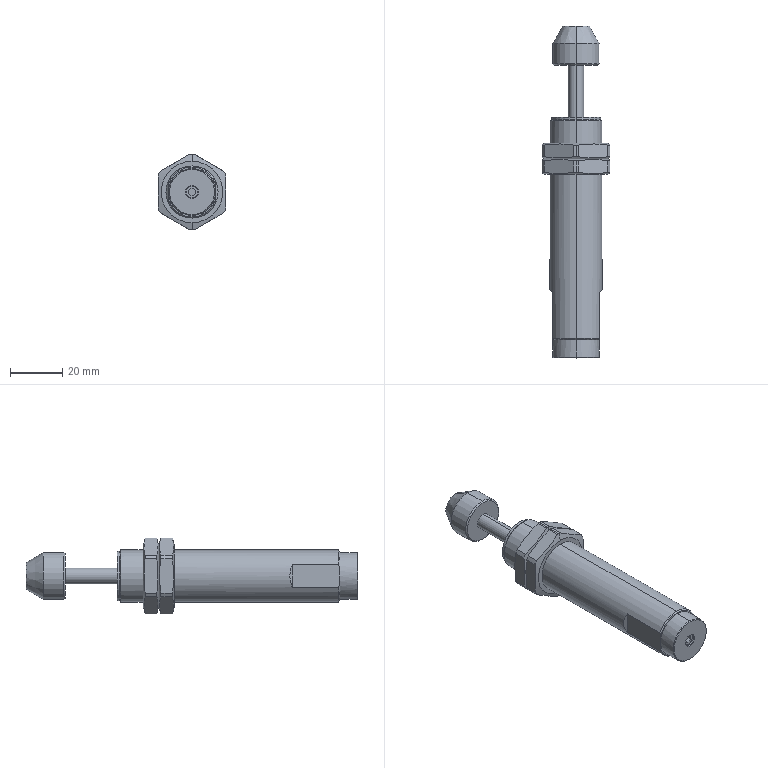Part | STEP file | 11-ACA2020-311 | 3 solids | 96 faces | box 26 x 127.5 x 29.132 mm | volume 35458 mm3 | plane 35 | cone 31 | cylinder 30 | commonest cylinder face diameters 29.132 x14 18 x4 19.188 x4 4.459 x2 6 x2 19 x2